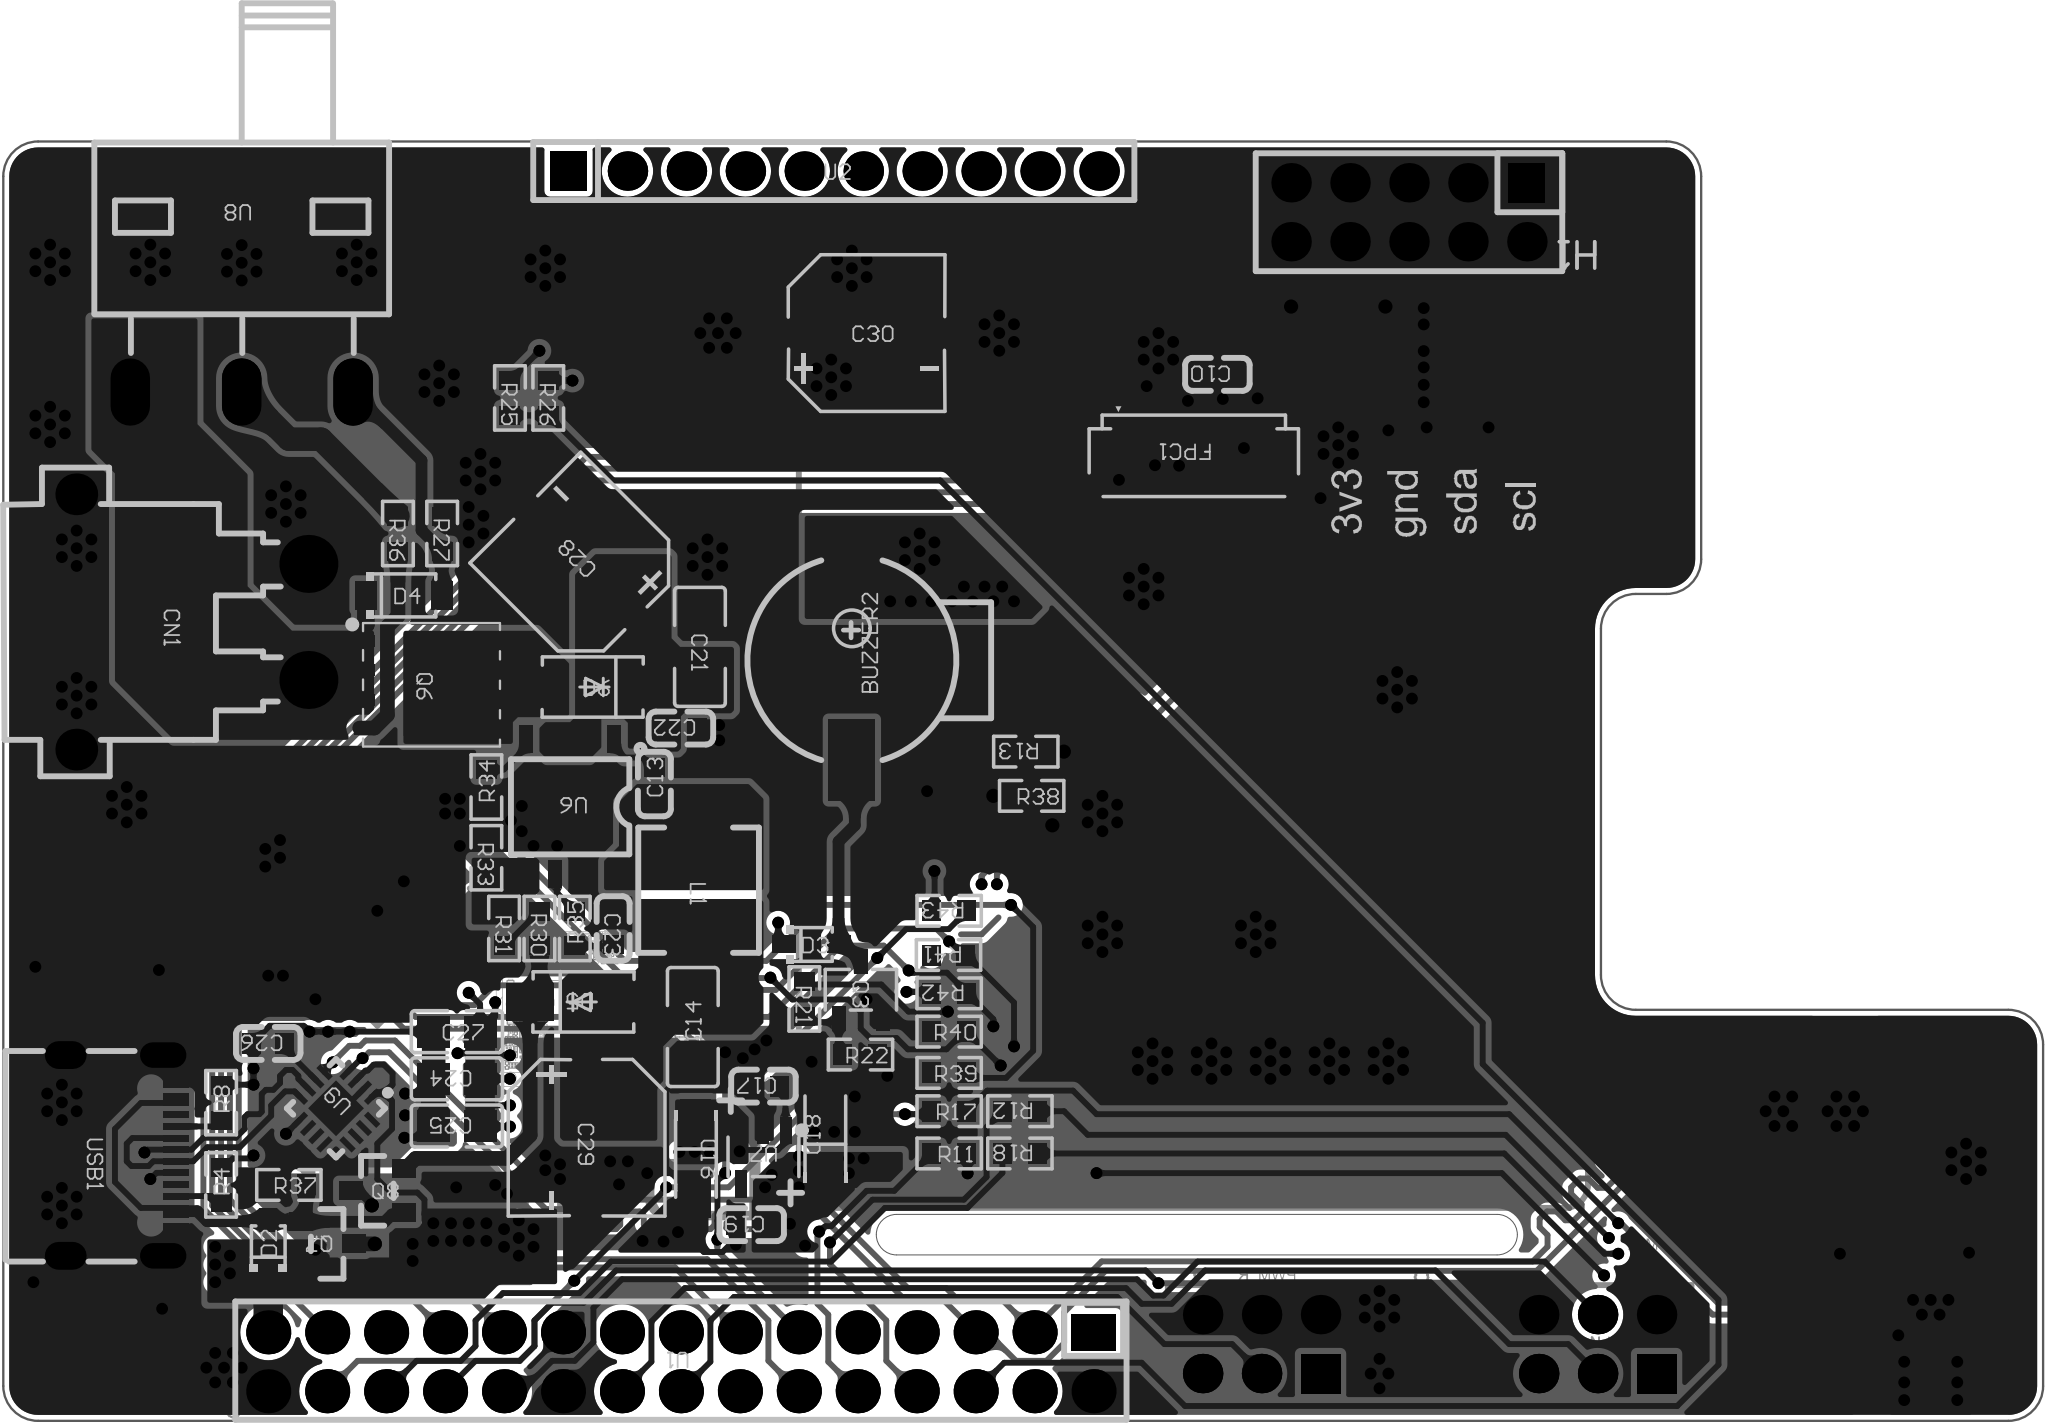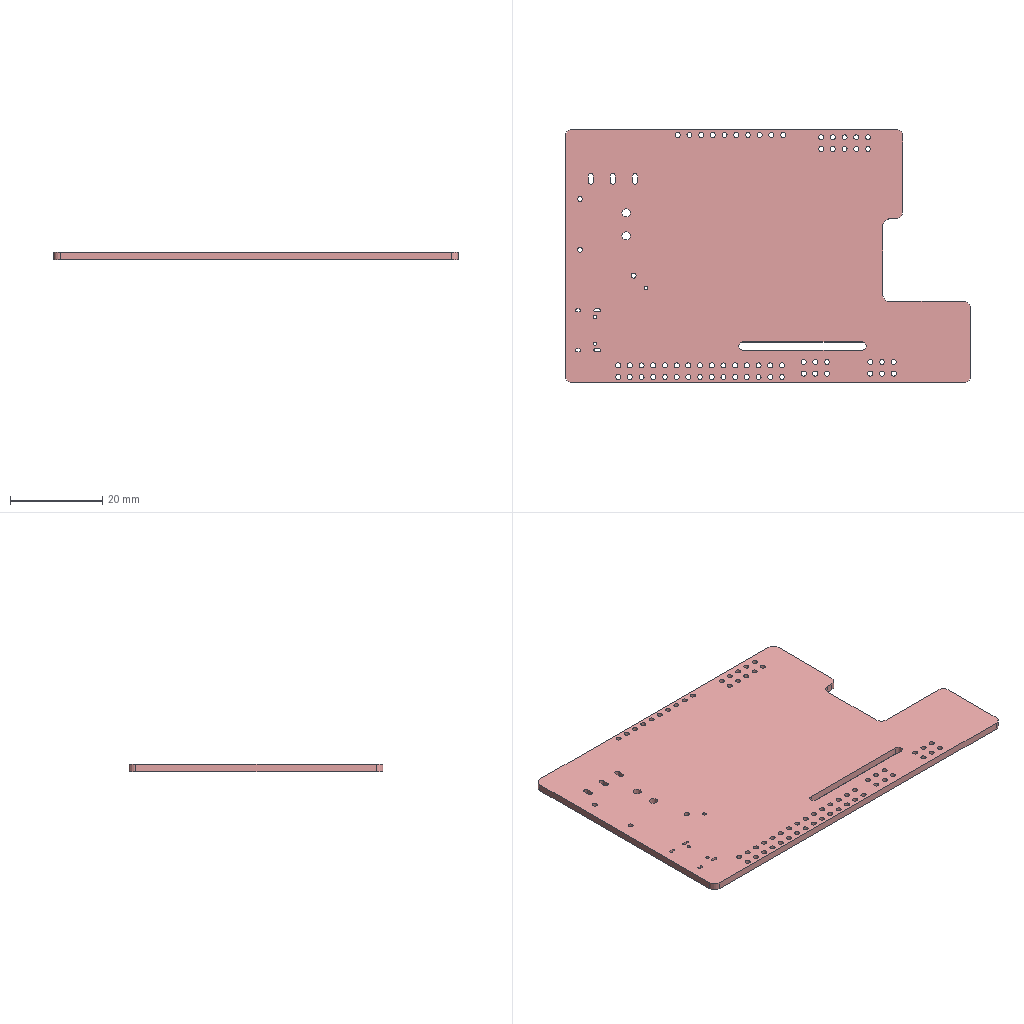Circuit board layout | Altium Designer | box 87.9 x 55.1 x 1.6 mm
Layer stack:
# Altium Designer layer stack of  (unit mm; dielectric type: 0 none, 1 core, 2 prepreg, 3 surface material)
index,name,kind,layer,copper_thickness_mm,dielectric_type,dielectric_thickness_mm,dielectric_material,dielectric_constant
0,Top Paste Mask Layer,other,,,,,,
1,Top Silkscreen Layer,other,,,,,,
2,Top Solder Mask Layer,dielectric,,,3,0,,0
3,Top Layer,copper,Top Layer,0.035,,,,
4,Dielectric1,dielectric,,,3,0.2104,7628 RC49% 8.6mil,0
5,VCC,copper,VCC,0.0152,,,,
6,Dielectric2,dielectric,,,3,1.065,1.1mm H/HOZ Copper,0
7,GND,copper,GND,0.0152,,,,
8,Dielectric3,dielectric,,,3,0.2104,7628 RC49% 8.6mil,0
9,Bottom Layer,copper,Bottom Layer,0.035,,,,
10,Bottom Solder Mask Layer,dielectric,,,3,0,,0
11,Bottom Silkscreen Layer,other,,,,,,
12,Bottom Paste Mask Layer,other,,,,,,
# drill layer pairs: low layer,high layer
drill_pair,Top Layer,Bottom Layer
Part placement:
Designator,Comment,Layer,Footprint,Center-X(mm),Center-Y(mm),Rotation
C30,100uF,TopLayer,CAP-SMD_BD6.3-L6.6-W6.6-FD-1,114.427,125.095,0
R36,10Ω,TopLayer,R0603,94.234,116.459,270
C21,4.7uF,TopLayer,C1206,107.246,111.575,270
C22,100nF,TopLayer,C0603,106.426,108.077,180
C23,4.7nF,TopLayer,C0603,103.505,99.441,270
C14,47uF,TopLayer,C1206,106.939,95.195,90
C16,10uF,TopLayer,CAP-SMD_L3.2-W1.6-RD-C7171,107.073,89.535,270
C17,100nF,TopLayer,C0603,109.982,92.65,180
C18,10uF,TopLayer,CAP-SMD_L3.2-W1.6-RD-C7171,112.649,90.551,90
C19,100nF,TopLayer,C0603,109.474,86.68,180
C13,100nF,TopLayer,C0603,105.283,105.664,90
C28,100uF,TopLayer,CAP-SMD_BD6.3-L6.6-W6.6-FD-1,102.108,115.189,135
C29,220uF,TopLayer,CAP-SMD_BD6.3-L6.6-W6.6-LS7.3-FD-H7.7,102.362,90.424,270
Q6,CJAC70P06,TopLayer,TDSON-8_L5.9-W5.2-P1.27-BL,94.694,109.941,270
H11,HX PZ2.54-2x3P TP,BottomLayer,HDR-SMD_6P-P2.54-V-M-R2-C3-LS7.2_M20-8760342,160.274,82.804,180
C10,100nF,TopLayer,C0603,129.54,123.317,180
U8,SS12D10G6-WJ,TopLayer,SW-TH_3P-P4.80_HX-SS12D10G6-WJ,87.503,122.555,180
H12,HX PZ2.54-2x3P TP,BottomLayer,HDR-SMD_6P-P2.54-V-M-R2-C3-LS7.2_M20-8760342,105.41,125.095,180
CN1,XT30PW-M30.G.Y,TopLayer,CONN-TH_XT30PW-M,85.376,112.649,270
D4,BZT52C16,TopLayer,SOD-123_L2.7-W1.6-LS3.7-RD,94.488,113.792,0
D5,SS54,TopLayer,SMA_L4.3-W2.6-LS5.0-FD,102.235,96.266,180
D6,SS54,TopLayer,SMA_L4.3-W2.6-LS5.0-FD,102.616,109.855,0
D3,1N5819WS,TopLayer,SOD-323_L1.8-W1.3-LS2.5-RD,112.045,98.752,0
D2,1N5819WS,TopLayer,SOD-323_L1.8-W1.3-LS2.5-RD,88.646,85.725,90
FPC1,HC-FPC-05-09-14RLTAG,TopLayer,FPC-SMD_14P-P0.50_HC-FPC-05-09-14RLTAG,128.524,119.761,180
L1,4.7uH,TopLayer,IND-SMD_L5.4-W5.2_FXL0530,107.188,101.092,270
LED4,NCD0603R1,BottomLayer,LED0603-RD_RED,79.138,96.648,0
LED3,NCD0603R1,BottomLayer,LED0603-RD_RED,79.265,83.059,0
Q3,S8050,TopLayer,SOT-23-3_L2.9-W1.6-P1.90-LS2.8-BR,114.18,96.802,270
R27,10kΩ,TopLayer,R0603,96.139,116.459,270
R34,200kΩ,TopLayer,R0603,98.044,105.537,90
R35,20kΩ,TopLayer,R0603,101.854,99.441,90
R30,51kΩ,TopLayer,R0603,100.33,99.441,270
R31,1.5kΩ,TopLayer,R0603,98.806,99.441,270
R33,10kΩ,TopLayer,R0603,98.044,102.489,270
R29,4.7kΩ,BottomLayer,R0603,82.272,83.046,0
R32,2.7kΩ,BottomLayer,R0603,82.145,96.635,180
R4,5.1kΩ,TopLayer,R0603,86.614,88.392,90
R8,5.1kΩ,TopLayer,R0603,86.614,91.936,90
R9,0Ω,BottomLayer,R1206,89.281,94.615,90
R22,10kΩ,TopLayer,R0603,114.162,94.008,0
R21,1kΩ,TopLayer,R0603,111.743,96.405,270
Q7,AO3401A,TopLayer,SOT-23_L2.9-W1.3-P1.90-LS2.4-BR,91.186,85.852,180
R11,100Ω,TopLayer,R0603,117.983,89.747,0
R17,100Ω,TopLayer,R0603,117.983,91.568,0
R12,100Ω,TopLayer,R0603,121.031,91.568,180
R18,100Ω,TopLayer,R0603,121.031,89.747,180
R25,100Ω,TopLayer,R0603,99.06,122.301,270
R26,100Ω,TopLayer,R0603,100.711,122.301,270
R13,5.1kΩ,TopLayer,R0603,121.285,107.061,180
R38,5.1kΩ,TopLayer,R0603,121.539,105.156,0
U6,SCT2450STER,TopLayer,ESOP-8_L4.9-W3.9-P1.27-LS6.0-BL-EP,101.654,104.684,180
U7,RT9013-33GB,TopLayer,SOT-23-5_L3.0-W1.7-P0.95-LS2.8-BL,109.982,89.602,180
USB1,TYPE-C 16PIN 2MD(073),TopLayer,USB-C-SMD_TYPE-C-6PIN-2MD-073,82.296,89.662,270
U1,2541FV-2x15P-B,TopLayer,HDR-TH_30P-P2.54-V-F-R2-C15-S2.54,106.426,80.772,180
U2,PM2.54-1*10,TopLayer,HDR-TH_10P-P2.54-V-F,113.013,132.077,0
U13,5BME8-08872-204-W0,BottomLayer,CONN-SMD_5BME8-08872-204-W0,152.781,91.186,0
H14,PZ254V-12-6P,BottomLayer,HDR-TH_6P-P2.54-V-M-R2-C3-S2.54,131.445,81.534,180
R39,10kΩ,TopLayer,R0603,117.983,93.218,0
Q8,AO3401A,TopLayer,SOT-23_L2.9-W1.3-P1.90-LS2.4-BR,93.345,88.138,0
R37,10kΩ,TopLayer,R0603,89.535,88.392,0
R40,10kΩ,TopLayer,R0603,117.983,94.996,0
R41,10kΩ,TopLayer,R0603,117.955,98.298,180
R42,10kΩ,TopLayer,R0603,117.983,96.647,180
R43,10kΩ,TopLayer,R0603,117.983,100.203,180
SW1,7*7*5-6P-L WX,BottomLayer,SW-SMD_8P-L7.0-W7.0-P1.40-LS7.4-TL,93.345,100.203,225
C24,1uF,TopLayer,C0805,96.774,92.964,180
C25,1uF,TopLayer,C0805,96.774,90.932,180
C26,100nF,TopLayer,C0603,88.646,94.488,180
C27,1uF,TopLayer,C0805,96.774,94.996,0
U9,CH343P,TopLayer,TQFN-16_L3.0-W3.0-P0.50-BL-EP1.7,91.567,91.695,135
BUZZER2,2.7kHz,TopLayer,BUZ-SMD_GSC9032RB,113.792,110.998,90
H13,PZ254V-12-6P,BottomLayer,HDR-TH_6P-P2.54-V-M-R2-C3-S2.54,145.923,81.534,180
H1,,TopLayer,HDR-TH_10P-P2.54-V-F-R2-C5-S2.54,137.795,130.302,180
Pad and via stacks:
# Altium Designer via and pad stacks of  (unit mm). Each distinct definition once, with the count of objects using it.
# via: kind,start_layer,end_layer,hole_mm,diameter_mm,mode(0 simple;1 top-mid-bottom;2 full stack),diameter_per_layer,count,example_net
# pad: kind,layer,hole_mm,hole_type(0 round;1 square;2 slot),plating,top_size,top_shape(1 round;2 rect;3 octagon;9 rounded rect),mid_size,bottom_size,mode,footprint,size_per_layer,count,example
pad,Top Layer,0,0,plated,3.8x1.2,2,3.8x1.2,3.8x1.2,0,CAP-SMD_BD6.3-L6.6-W6.6-FD-1,,4,C30.1
pad,Top Layer,0,0,plated,0.8065x0.864,2,0.8065x0.864,0.8065x0.864,0,R0603,,50,R36.2
pad,Top Layer,0,0,plated,1.485x1.728,2,1.485x1.728,1.485x1.728,0,C1206,,4,C21.2
pad,Top Layer,0,0,plated,0.8x0.9,2,0.8x0.9,0.8x0.9,0,C0603,,14,C22.2
pad,Top Layer,0,0,plated,1.758x1.296,2,1.758x1.296,1.758x1.296,0,CAP-SMD_L3.2-W1.6-RD-C7171,,4,C16.1
pad,Top Layer,0,0,plated,3.5x1.2,2,3.5x1.2,3.5x1.2,0,CAP-SMD_BD6.3-L6.6-W6.6-LS7.3-FD-H7.7,,2,C29.1
pad,Top Layer,0,0,plated,0.5x0.9,2,0.5x0.9,0.5x0.9,0,TDSON-8_L5.9-W5.2-P1.27-BL,,4,Q6.1
pad,Top Layer,0,0,plated,1.638x1.638,1,1.638x1.638,1.638x1.638,0,TDSON-8_L5.9-W5.2-P1.27-BL,,1,Q6.5
pad,Top Layer,0,0,plated,0.91x1.22,2,0.91x1.22,0.91x1.22,0,SOD-123_L2.7-W1.6-LS3.7-RD,,2,D4.2
pad,Top Layer,0,0,plated,2.046x1.62,2,2.046x1.62,2.046x1.62,0,SMA_L4.3-W2.6-LS5.0-FD,,4,D5.1
pad,Top Layer,0,0,plated,1x0.75,2,1x0.75,1x0.75,0,SOD-323_L1.8-W1.3-LS2.5-RD,,4,D3.2
pad,Top Layer,0,0,plated,0.3x0.8,2,0.3x0.8,0.3x0.8,0,FPC-SMD_14P-P0.50_HC-FPC-05-09-14RLTAG,,14,FPC1.1
pad,Top Layer,0,0,plated,0.4x0.8,2,0.4x0.8,0.4x0.8,0,FPC-SMD_14P-P0.50_HC-FPC-05-09-14RLTAG,,2,FPC1.16
pad,Top Layer,0,0,plated,1.9x2.5,2,1.9x2.5,1.9x2.5,0,IND-SMD_L5.4-W5.2_FXL0530,,2,L1.1
pad,Top Layer,0,0,plated,1.07x0.6,2,1.07x0.6,1.07x0.6,0,SOT-23-3_L2.9-W1.6-P1.90-LS2.8-BR,,3,Q3.1
pad,Top Layer,0,0,plated,1x0.8,2,1x0.8,1x0.8,0,SOT-23_L2.9-W1.3-P1.90-LS2.4-BR,,6,Q7.2
pad,Top Layer,0,0,plated,0.6x1.2,2,0.6x1.2,0.6x1.2,0,ESOP-8_L4.9-W3.9-P1.27-LS6.0-BL-EP,,8,U6.1
pad,Top Layer,0,0,plated,3.3x2.4,2,3.3x2.4,3.3x2.4,0,ESOP-8_L4.9-W3.9-P1.27-LS6.0-BL-EP,,1,U6.9
pad,Top Layer,0,0,plated,0.49x1.157,2,0.49x1.157,0.49x1.157,0,SOT-23-5_L3.0-W1.7-P0.95-LS2.8-BL,,3,U7.1
pad,Top Layer,0,0,plated,0.49x1.175,2,0.49x1.175,0.49x1.175,0,SOT-23-5_L3.0-W1.7-P0.95-LS2.8-BL,,2,U7.4
pad,Top Layer,0,0,plated,0.55x1.1,2,0.55x1.1,0.55x1.1,0,USB-C-SMD_TYPE-C-6PIN-2MD-073,,4,USB1.1
pad,Top Layer,0,0,plated,0.3x1.1,2,0.3x1.1,0.3x1.1,0,USB-C-SMD_TYPE-C-6PIN-2MD-073,,8,USB1.3
pad,Top Layer,0,0,plated,1.41x1.35,2,1.41x1.35,1.41x1.35,0,C0805,,6,C24.2
pad,Top Layer,0,0,plated,0.25x0.75,2,0.25x0.75,0.25x0.75,0,TQFN-16_L3.0-W3.0-P0.50-BL-EP1.7,,8,U9.1
pad,Top Layer,0,0,plated,0.75x0.25,2,0.75x0.25,0.75x0.25,0,TQFN-16_L3.0-W3.0-P0.50-BL-EP1.7,,8,U9.5
pad,Top Layer,0,0,plated,1.7x1.7,2,1.7x1.7,1.7x1.7,0,TQFN-16_L3.0-W3.0-P0.50-BL-EP1.7,,1,U9.17
pad,Top Layer,0,0,plated,3.5x2,2,3.5x2,3.5x2,0,BUZ-SMD_GSC9032RB,,2,BUZZER2.1
pad,Bottom Layer,0,0,plated,1.02x3,2,1.02x3,1.02x3,0,HDR-SMD_6P-P2.54-V-M-R2-C3-LS7.2_M20-8760342,,12,H11.1
pad,Bottom Layer,0,0,plated,0.8x0.8,2,0.8x0.8,0.8x0.8,0,LED0603-RD_RED,,4,LED4.1
pad,Bottom Layer,0,0,plated,0.8065x0.864,2,0.8065x0.864,0.8065x0.864,0,R0603,,4,R29.2
pad,Bottom Layer,0,0,plated,1.208x1.701,2,1.208x1.701,1.208x1.701,0,R1206,,2,R9.2
pad,Bottom Layer,0,0,plated,1.02x2.5,2,1.02x2.5,1.02x2.5,0,CONN-SMD_5BME8-08872-204-W0,,8,U13.1
pad,Bottom Layer,0,0,plated,1.5x1,2,1.5x1,1.5x1,0,SW-SMD_8P-L7.0-W7.0-P1.40-LS7.4-TL,,8,SW1.1
pad,Multi-Layer,1.1,2,plated,1.7x2.9,1,1.7x2.9,1.7x2.9,0,SW-TH_3P-P4.80_HX-SS12D10G6-WJ,,3,U8.3
pad,Multi-Layer,1.8,0,plated,2.5x2.5,1,2.5x2.5,2.5x2.5,0,CONN-TH_XT30PW-M,,2,CN1.1
pad,Multi-Layer,1.1,0,plated,1.8x1.8,1,1.8x1.8,1.8x1.8,0,CONN-TH_XT30PW-M,,2,CN1.3
pad,Multi-Layer,0.6,2,plated,1.1x2,1,1.1x2,1.1x2,0,USB-C-SMD_TYPE-C-6PIN-2MD-073,,2,USB1.13
pad,Multi-Layer,0.6,2,plated,1.2x1.8,1,1.2x1.8,1.2x1.8,0,USB-C-SMD_TYPE-C-6PIN-2MD-073,,2,USB1.13
pad,Multi-Layer,1.1,0,plated,1.9x1.575,2,1.9x1.575,1.9x1.575,0,HDR-TH_30P-P2.54-V-F-R2-C15-S2.54,,1,U1.1
pad,Multi-Layer,1.1,0,plated,1.9x1.9,1,1.9x1.9,1.9x1.9,0,HDR-TH_30P-P2.54-V-F-R2-C15-S2.54,,29,U1.2
pad,Multi-Layer,1.1,0,plated,1.7x1.7,1,1.7x1.7,1.7x1.7,0,HDR-TH_10P-P2.54-V-F,,9,U2.10
pad,Multi-Layer,1.1,0,plated,1.575x1.7,2,1.575x1.7,1.575x1.7,0,HDR-TH_10P-P2.54-V-F,,1,U2.1
pad,Multi-Layer,1.1,0,plated,1.7x1.7,2,1.7x1.7,1.7x1.7,0,HDR-TH_6P-P2.54-V-M-R2-C3-S2.54,,2,H14.1
pad,Multi-Layer,1.1,0,plated,1.7x1.7,1,1.7x1.7,1.7x1.7,0,HDR-TH_6P-P2.54-V-M-R2-C3-S2.54,,10,H14.2
pad,Multi-Layer,1.1,0,plated,1.7x1.7,1,1.7x1.7,1.7x1.7,0,HDR-TH_10P-P2.54-V-F-R2-C5-S2.54,,9,H1.10
pad,Multi-Layer,1.1,0,plated,1.575x1.7,2,1.575x1.7,1.575x1.7,0,HDR-TH_10P-P2.54-V-F-R2-C5-S2.54,,1,H1.1
via,Top Layer,Bottom Layer,0.3048,0.508,0,,455,+5V
via,Top Layer,Bottom Layer,0.3048,0.61,0,,7,I2C_SCL
Copper pours:
name,layer,net,type(0 solid;1 hatched;2 none)
Bottom Layer-+5V,Bottom Layer,+5V,0
Bottom Layer-AGND,Bottom Layer,AGND,0
Bottom Layer-GND,Bottom Layer,GND,0
Top Layer-3V3,Top Layer,3V3,0
Top Layer-+5V,Top Layer,+5V,0
Top Layer-GND,Top Layer,GND,0
Top Layer-VCCBAT,Top Layer,VCCBAT,0
Top Layer-GND 1,Top Layer,GND,0
Top Layer-$2N1742,Top Layer,$2N1742,0
Top Layer-$2N1744,Top Layer,$2N1744,0
Top Layer-+5V 1,Top Layer,+5V,0
Top Layer-$2N1752,Top Layer,$2N1752,0
Top Layer-$2N1748,Top Layer,$2N1748,0
Top Layer-+5V 2,Top Layer,+5V,0
Top Layer-+5V 3,Top Layer,+5V,0
Top Layer-3V3 1,Top Layer,3V3,0
Top Layer-$1N4144,Top Layer,$1N4144,0
GND-AGND,GND,AGND,0
GND-AGND 1,GND,AGND,0
GND-GND,GND,GND,0
Design rules, without the lines most boards share:
# Altium Designer design rules of  (exported by Altium Designer, unit mm)
# columns: name | kind | enabled | priority | scope1 | scope2 | descriptor | typed fields (field=value)
innerPlane | 6 | enabled | 1 | All | All | Power Plane Connect Rule(Direct Connect )(Expansion=20mil) (Conductor Width=10mil) (Air Gap=10mil) (Entries=4) (All) | relief_conductor_width=0.254 relief_entries=4 relief_expansion=0.508
copperRegion | 20 | enabled | 1 | All | All | Polygon Connect Rule(Direct Connect )(Conductor Width=10mil) (Relief Angle=90 Angle) (Entries=4) (Air Gap Width=10mil) (All),(All) | connect_style(0=relief,1=direct,2=none)=1 relief_conductor_width=0.254 relief_entries=4
solderMaskExpansion | 13 | enabled | 2 | All | All | Solder Mask Expansion (Expansion =2.008mil) (All) | expansion=0.051